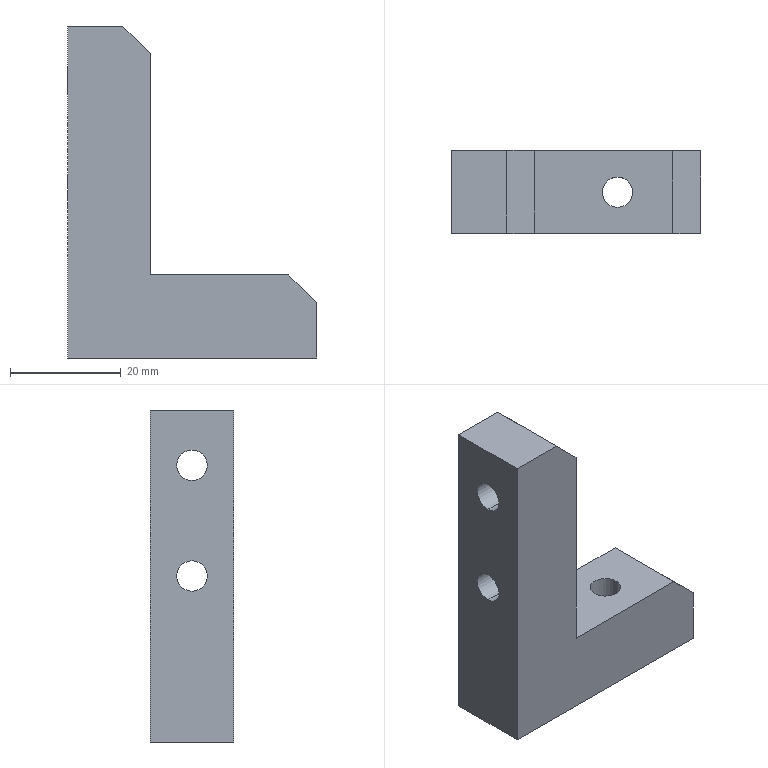Part | SolidWorks | features HoleWzd 2, Chamfer 1, Extrusion 1 | 1 solid | 16 faces | box 45 x 15 x 60 mm | volume 18806 mm3 | plane 10 | cylinder 6 | commonest cylinder face diameters 5.5 x6
STEP:
#1=CARTESIAN_POINT('',(12.25,0.,-15.));
#2=VERTEX_POINT('',#1);
#3=CARTESIAN_POINT('',(17.75,0.,-15.));
#4=VERTEX_POINT('',#3);
#5=CARTESIAN_POINT('',(15.,0.,-15.));
#6=DIRECTION('',(0.,0.,1.));
#7=DIRECTION('',(1.,0.,0.));
#8=AXIS2_PLACEMENT_3D('',#5,#6,#7);
#9=CIRCLE('',#8,2.75);
#10=EDGE_CURVE('',#2,#4,#9,.T.);
#11=ORIENTED_EDGE('',*,*,#10,.F.);
#12=CARTESIAN_POINT('',(12.25,0.,0.));
#13=VERTEX_POINT('',#12);
#14=CARTESIAN_POINT('',(12.25,0.,0.));
#15=DIRECTION('',(0.,0.,1.));
#16=VECTOR('',#15,1000.);
#17=LINE('',#14,#16);
#18=EDGE_CURVE('',#2,#13,#17,.T.);
#19=ORIENTED_EDGE('',*,*,#18,.T.);
#20=CARTESIAN_POINT('',(17.75,0.,0.));
#21=VERTEX_POINT('',#20);
#22=CARTESIAN_POINT('',(15.,0.,0.));
#23=DIRECTION('',(0.,0.,1.));
#24=DIRECTION('',(1.,0.,0.));
#25=AXIS2_PLACEMENT_3D('',#22,#23,#24);
#26=CIRCLE('',#25,2.75);
#27=EDGE_CURVE('',#13,#21,#26,.T.);
#28=ORIENTED_EDGE('',*,*,#27,.T.);
#29=CARTESIAN_POINT('',(17.75,0.,0.));
#30=DIRECTION('',(0.,0.,1.));
#31=VECTOR('',#30,1000.);
#32=LINE('',#29,#31);
#33=EDGE_CURVE('',#4,#21,#32,.T.);
#34=ORIENTED_EDGE('',*,*,#33,.F.);
#35=EDGE_LOOP('',(#11,#19,#28,#34));
#36=FACE_OUTER_BOUND('',#35,.T.);
#37=CARTESIAN_POINT('',(15.,0.,0.));
#38=DIRECTION('',(0.,0.,1.));
#39=DIRECTION('',(1.,0.,0.));
#40=AXIS2_PLACEMENT_3D('',#37,#38,#39);
#41=CYLINDRICAL_SURFACE('',#40,2.75);
#42=ADVANCED_FACE('',(#36),#41,.F.);
#43=CARTESIAN_POINT('',(-15.,0.,37.75));
#44=VERTEX_POINT('',#43);
#45=CARTESIAN_POINT('',(-15.,0.,32.25));
#46=VERTEX_POINT('',#45);
#47=CARTESIAN_POINT('',(-15.,0.,35.));
#48=DIRECTION('',(1.,0.,0.));
#49=DIRECTION('',(0.,0.,-1.));
#50=AXIS2_PLACEMENT_3D('',#47,#48,#49);
#51=CIRCLE('',#50,2.75);
#52=EDGE_CURVE('',#44,#46,#51,.T.);
#53=ORIENTED_EDGE('',*,*,#52,.F.);
#54=CARTESIAN_POINT('',(0.,0.,37.75));
#55=VERTEX_POINT('',#54);
#56=CARTESIAN_POINT('',(0.,0.,37.75));
#57=DIRECTION('',(1.,0.,0.));
#58=VECTOR('',#57,1000.);
#59=LINE('',#56,#58);
#60=EDGE_CURVE('',#44,#55,#59,.T.);
#61=ORIENTED_EDGE('',*,*,#60,.T.);
#62=CARTESIAN_POINT('',(0.,0.,32.25));
#63=VERTEX_POINT('',#62);
#64=CARTESIAN_POINT('',(0.,0.,35.));
#65=DIRECTION('',(1.,0.,0.));
#66=DIRECTION('',(0.,0.,-1.));
#67=AXIS2_PLACEMENT_3D('',#64,#65,#66);
#68=CIRCLE('',#67,2.75);
#69=EDGE_CURVE('',#55,#63,#68,.T.);
#70=ORIENTED_EDGE('',*,*,#69,.T.);
#71=CARTESIAN_POINT('',(0.,0.,32.25));
#72=DIRECTION('',(1.,0.,0.));
#73=VECTOR('',#72,1000.);
#74=LINE('',#71,#73);
#75=EDGE_CURVE('',#46,#63,#74,.T.);
#76=ORIENTED_EDGE('',*,*,#75,.F.);
#77=EDGE_LOOP('',(#53,#61,#70,#76));
#78=FACE_OUTER_BOUND('',#77,.T.);
#79=CARTESIAN_POINT('',(0.,0.,35.));
#80=DIRECTION('',(1.,0.,0.));
#81=DIRECTION('',(0.,0.,-1.));
#82=AXIS2_PLACEMENT_3D('',#79,#80,#81);
#83=CYLINDRICAL_SURFACE('',#82,2.75);
#84=ADVANCED_FACE('',(#78),#83,.F.);
#85=CARTESIAN_POINT('',(-15.,0.,17.75));
#86=VERTEX_POINT('',#85);
#87=CARTESIAN_POINT('',(-15.,0.,12.25));
#88=VERTEX_POINT('',#87);
#89=CARTESIAN_POINT('',(-15.,0.,15.));
#90=DIRECTION('',(1.,0.,0.));
#91=DIRECTION('',(0.,0.,-1.));
#92=AXIS2_PLACEMENT_3D('',#89,#90,#91);
#93=CIRCLE('',#92,2.75);
#94=EDGE_CURVE('',#86,#88,#93,.T.);
#95=ORIENTED_EDGE('',*,*,#94,.F.);
#96=CARTESIAN_POINT('',(0.,0.,17.75));
#97=VERTEX_POINT('',#96);
#98=CARTESIAN_POINT('',(0.,0.,17.75));
#99=DIRECTION('',(1.,0.,0.));
#100=VECTOR('',#99,1000.);
#101=LINE('',#98,#100);
#102=EDGE_CURVE('',#86,#97,#101,.T.);
#103=ORIENTED_EDGE('',*,*,#102,.T.);
#104=CARTESIAN_POINT('',(0.,0.,12.25));
#105=VERTEX_POINT('',#104);
#106=CARTESIAN_POINT('',(0.,0.,15.));
#107=DIRECTION('',(1.,0.,0.));
#108=DIRECTION('',(0.,0.,-1.));
#109=AXIS2_PLACEMENT_3D('',#106,#107,#108);
#110=CIRCLE('',#109,2.75);
#111=EDGE_CURVE('',#97,#105,#110,.T.);
#112=ORIENTED_EDGE('',*,*,#111,.T.);
#113=CARTESIAN_POINT('',(0.,0.,12.25));
#114=DIRECTION('',(1.,0.,0.));
#115=VECTOR('',#114,1000.);
#116=LINE('',#113,#115);
#117=EDGE_CURVE('',#88,#105,#116,.T.);
#118=ORIENTED_EDGE('',*,*,#117,.F.);
#119=EDGE_LOOP('',(#95,#103,#112,#118));
#120=FACE_OUTER_BOUND('',#119,.T.);
#121=CARTESIAN_POINT('',(0.,0.,15.));
#122=DIRECTION('',(1.,0.,0.));
#123=DIRECTION('',(0.,0.,-1.));
#124=AXIS2_PLACEMENT_3D('',#121,#122,#123);
#125=CYLINDRICAL_SURFACE('',#124,2.75);
#126=ADVANCED_FACE('',(#120),#125,.F.);
#127=CARTESIAN_POINT('',(-15.,0.,35.));
#128=DIRECTION('',(1.,0.,0.));
#129=DIRECTION('',(0.,0.,-1.));
#130=AXIS2_PLACEMENT_3D('',#127,#128,#129);
#131=CIRCLE('',#130,2.75);
#132=EDGE_CURVE('',#46,#44,#131,.T.);
#133=ORIENTED_EDGE('',*,*,#132,.T.);
#134=ORIENTED_EDGE('',*,*,#52,.T.);
#135=EDGE_LOOP('',(#133,#134));
#136=FACE_BOUND('',#135,.T.);
#137=CARTESIAN_POINT('',(-15.,0.,15.));
#138=DIRECTION('',(1.,0.,0.));
#139=DIRECTION('',(0.,0.,-1.));
#140=AXIS2_PLACEMENT_3D('',#137,#138,#139);
#141=CIRCLE('',#140,2.75);
#142=EDGE_CURVE('',#88,#86,#141,.T.);
#143=ORIENTED_EDGE('',*,*,#142,.T.);
#144=ORIENTED_EDGE('',*,*,#94,.T.);
#145=EDGE_LOOP('',(#143,#144));
#146=FACE_BOUND('',#145,.T.);
#147=CARTESIAN_POINT('',(-15.,-7.5,-15.));
#148=VERTEX_POINT('',#147);
#149=CARTESIAN_POINT('',(-15.,-7.5,45.));
#150=VERTEX_POINT('',#149);
#151=CARTESIAN_POINT('',(-15.,-7.5,-15.));
#152=DIRECTION('',(0.,0.,1.));
#153=VECTOR('',#152,1000.);
#154=LINE('',#151,#153);
#155=EDGE_CURVE('',#148,#150,#154,.T.);
#156=ORIENTED_EDGE('',*,*,#155,.T.);
#157=CARTESIAN_POINT('',(-15.,7.5,45.));
#158=VERTEX_POINT('',#157);
#159=CARTESIAN_POINT('',(-15.,7.5,45.));
#160=DIRECTION('',(0.,-1.,0.));
#161=VECTOR('',#160,1000.);
#162=LINE('',#159,#161);
#163=EDGE_CURVE('',#158,#150,#162,.T.);
#164=ORIENTED_EDGE('',*,*,#163,.F.);
#165=CARTESIAN_POINT('',(-15.,7.5,-15.));
#166=VERTEX_POINT('',#165);
#167=CARTESIAN_POINT('',(-15.,7.5,-15.));
#168=DIRECTION('',(0.,0.,1.));
#169=VECTOR('',#168,1000.);
#170=LINE('',#167,#169);
#171=EDGE_CURVE('',#166,#158,#170,.T.);
#172=ORIENTED_EDGE('',*,*,#171,.F.);
#173=CARTESIAN_POINT('',(-15.,7.5,-15.));
#174=DIRECTION('',(0.,-1.,0.));
#175=VECTOR('',#174,1000.);
#176=LINE('',#173,#175);
#177=EDGE_CURVE('',#166,#148,#176,.T.);
#178=ORIENTED_EDGE('',*,*,#177,.T.);
#179=EDGE_LOOP('',(#156,#164,#172,#178));
#180=FACE_OUTER_BOUND('',#179,.T.);
#181=CARTESIAN_POINT('',(-15.,7.5,-15.));
#182=DIRECTION('',(1.,0.,0.));
#183=DIRECTION('',(0.,0.,-1.));
#184=AXIS2_PLACEMENT_3D('',#181,#182,#183);
#185=PLANE('',#184);
#186=ADVANCED_FACE('',(#136,#146,#180),#185,.F.);
#187=CARTESIAN_POINT('',(-5.,-7.5,45.));
#188=VERTEX_POINT('',#187);
#189=CARTESIAN_POINT('',(0.,-7.5,45.));
#190=DIRECTION('',(1.,0.,0.));
#191=VECTOR('',#190,1000.);
#192=LINE('',#189,#191);
#193=EDGE_CURVE('',#150,#188,#192,.T.);
#194=ORIENTED_EDGE('',*,*,#193,.T.);
#195=CARTESIAN_POINT('',(-5.,7.5,45.));
#196=VERTEX_POINT('',#195);
#197=CARTESIAN_POINT('',(-5.,7.5,45.));
#198=DIRECTION('',(0.,1.,0.));
#199=VECTOR('',#198,1000.);
#200=LINE('',#197,#199);
#201=EDGE_CURVE('',#188,#196,#200,.T.);
#202=ORIENTED_EDGE('',*,*,#201,.T.);
#203=CARTESIAN_POINT('',(0.,7.5,45.));
#204=DIRECTION('',(1.,0.,0.));
#205=VECTOR('',#204,1000.);
#206=LINE('',#203,#205);
#207=EDGE_CURVE('',#158,#196,#206,.T.);
#208=ORIENTED_EDGE('',*,*,#207,.F.);
#209=ORIENTED_EDGE('',*,*,#163,.T.);
#210=EDGE_LOOP('',(#194,#202,#208,#209));
#211=FACE_OUTER_BOUND('',#210,.T.);
#212=CARTESIAN_POINT('',(0.,7.5,45.));
#213=DIRECTION('',(0.,0.,-1.));
#214=DIRECTION('',(-1.,0.,0.));
#215=AXIS2_PLACEMENT_3D('',#212,#213,#214);
#216=PLANE('',#215);
#217=ADVANCED_FACE('',(#211),#216,.F.);
#218=CARTESIAN_POINT('',(0.,0.,35.));
#219=DIRECTION('',(1.,0.,0.));
#220=DIRECTION('',(0.,0.,-1.));
#221=AXIS2_PLACEMENT_3D('',#218,#219,#220);
#222=CIRCLE('',#221,2.75);
#223=EDGE_CURVE('',#63,#55,#222,.T.);
#224=ORIENTED_EDGE('',*,*,#223,.F.);
#225=ORIENTED_EDGE('',*,*,#69,.F.);
#226=EDGE_LOOP('',(#224,#225));
#227=FACE_BOUND('',#226,.T.);
#228=CARTESIAN_POINT('',(0.,0.,15.));
#229=DIRECTION('',(1.,0.,0.));
#230=DIRECTION('',(0.,0.,-1.));
#231=AXIS2_PLACEMENT_3D('',#228,#229,#230);
#232=CIRCLE('',#231,2.75);
#233=EDGE_CURVE('',#105,#97,#232,.T.);
#234=ORIENTED_EDGE('',*,*,#233,.F.);
#235=ORIENTED_EDGE('',*,*,#111,.F.);
#236=EDGE_LOOP('',(#234,#235));
#237=FACE_BOUND('',#236,.T.);
#238=CARTESIAN_POINT('',(0.,7.5,40.));
#239=VERTEX_POINT('',#238);
#240=CARTESIAN_POINT('',(0.,7.5,0.));
#241=VERTEX_POINT('',#240);
#242=CARTESIAN_POINT('',(0.,7.5,0.));
#243=DIRECTION('',(0.,0.,-1.));
#244=VECTOR('',#243,1000.);
#245=LINE('',#242,#244);
#246=EDGE_CURVE('',#239,#241,#245,.T.);
#247=ORIENTED_EDGE('',*,*,#246,.F.);
#248=CARTESIAN_POINT('',(0.,-7.5,40.));
#249=VERTEX_POINT('',#248);
#250=CARTESIAN_POINT('',(0.,7.5,40.));
#251=DIRECTION('',(0.,-1.,0.));
#252=VECTOR('',#251,1000.);
#253=LINE('',#250,#252);
#254=EDGE_CURVE('',#239,#249,#253,.T.);
#255=ORIENTED_EDGE('',*,*,#254,.T.);
#256=CARTESIAN_POINT('',(0.,-7.5,0.));
#257=VERTEX_POINT('',#256);
#258=CARTESIAN_POINT('',(0.,-7.5,0.));
#259=DIRECTION('',(0.,0.,-1.));
#260=VECTOR('',#259,1000.);
#261=LINE('',#258,#260);
#262=EDGE_CURVE('',#249,#257,#261,.T.);
#263=ORIENTED_EDGE('',*,*,#262,.T.);
#264=CARTESIAN_POINT('',(0.,7.5,0.));
#265=DIRECTION('',(0.,-1.,0.));
#266=VECTOR('',#265,1000.);
#267=LINE('',#264,#266);
#268=EDGE_CURVE('',#241,#257,#267,.T.);
#269=ORIENTED_EDGE('',*,*,#268,.F.);
#270=EDGE_LOOP('',(#247,#255,#263,#269));
#271=FACE_OUTER_BOUND('',#270,.T.);
#272=CARTESIAN_POINT('',(0.,7.5,0.));
#273=DIRECTION('',(-1.,0.,0.));
#274=DIRECTION('',(0.,0.,1.));
#275=AXIS2_PLACEMENT_3D('',#272,#273,#274);
#276=PLANE('',#275);
#277=ADVANCED_FACE('',(#227,#237,#271),#276,.F.);
#278=CARTESIAN_POINT('',(15.,0.,0.));
#279=DIRECTION('',(0.,0.,1.));
#280=DIRECTION('',(1.,0.,0.));
#281=AXIS2_PLACEMENT_3D('',#278,#279,#280);
#282=CIRCLE('',#281,2.75);
#283=EDGE_CURVE('',#21,#13,#282,.T.);
#284=ORIENTED_EDGE('',*,*,#283,.F.);
#285=ORIENTED_EDGE('',*,*,#27,.F.);
#286=EDGE_LOOP('',(#284,#285));
#287=FACE_BOUND('',#286,.T.);
#288=CARTESIAN_POINT('',(25.,-7.5,0.));
#289=VERTEX_POINT('',#288);
#290=CARTESIAN_POINT('',(30.,-7.5,0.));
#291=DIRECTION('',(1.,0.,0.));
#292=VECTOR('',#291,1000.);
#293=LINE('',#290,#292);
#294=EDGE_CURVE('',#257,#289,#293,.T.);
#295=ORIENTED_EDGE('',*,*,#294,.T.);
#296=CARTESIAN_POINT('',(25.,7.5,0.));
#297=VERTEX_POINT('',#296);
#298=CARTESIAN_POINT('',(25.,7.5,0.));
#299=DIRECTION('',(0.,1.,0.));
#300=VECTOR('',#299,1000.);
#301=LINE('',#298,#300);
#302=EDGE_CURVE('',#289,#297,#301,.T.);
#303=ORIENTED_EDGE('',*,*,#302,.T.);
#304=CARTESIAN_POINT('',(30.,7.5,0.));
#305=DIRECTION('',(1.,0.,0.));
#306=VECTOR('',#305,1000.);
#307=LINE('',#304,#306);
#308=EDGE_CURVE('',#241,#297,#307,.T.);
#309=ORIENTED_EDGE('',*,*,#308,.F.);
#310=ORIENTED_EDGE('',*,*,#268,.T.);
#311=EDGE_LOOP('',(#295,#303,#309,#310));
#312=FACE_OUTER_BOUND('',#311,.T.);
#313=CARTESIAN_POINT('',(30.,7.5,0.));
#314=DIRECTION('',(0.,0.,-1.));
#315=DIRECTION('',(-1.,0.,0.));
#316=AXIS2_PLACEMENT_3D('',#313,#314,#315);
#317=PLANE('',#316);
#318=ADVANCED_FACE('',(#287,#312),#317,.F.);
#319=CARTESIAN_POINT('',(30.,7.5,-5.));
#320=VERTEX_POINT('',#319);
#321=CARTESIAN_POINT('',(30.,7.5,-15.));
#322=VERTEX_POINT('',#321);
#323=CARTESIAN_POINT('',(30.,7.5,-15.));
#324=DIRECTION('',(0.,0.,-1.));
#325=VECTOR('',#324,1000.);
#326=LINE('',#323,#325);
#327=EDGE_CURVE('',#320,#322,#326,.T.);
#328=ORIENTED_EDGE('',*,*,#327,.F.);
#329=CARTESIAN_POINT('',(30.,-7.5,-5.));
#330=VERTEX_POINT('',#329);
#331=CARTESIAN_POINT('',(30.,7.5,-5.));
#332=DIRECTION('',(0.,-1.,0.));
#333=VECTOR('',#332,1000.);
#334=LINE('',#331,#333);
#335=EDGE_CURVE('',#320,#330,#334,.T.);
#336=ORIENTED_EDGE('',*,*,#335,.T.);
#337=CARTESIAN_POINT('',(30.,-7.5,-15.));
#338=VERTEX_POINT('',#337);
#339=CARTESIAN_POINT('',(30.,-7.5,-15.));
#340=DIRECTION('',(0.,0.,-1.));
#341=VECTOR('',#340,1000.);
#342=LINE('',#339,#341);
#343=EDGE_CURVE('',#330,#338,#342,.T.);
#344=ORIENTED_EDGE('',*,*,#343,.T.);
#345=CARTESIAN_POINT('',(30.,7.5,-15.));
#346=DIRECTION('',(0.,-1.,0.));
#347=VECTOR('',#346,1000.);
#348=LINE('',#345,#347);
#349=EDGE_CURVE('',#322,#338,#348,.T.);
#350=ORIENTED_EDGE('',*,*,#349,.F.);
#351=EDGE_LOOP('',(#328,#336,#344,#350));
#352=FACE_OUTER_BOUND('',#351,.T.);
#353=CARTESIAN_POINT('',(30.,7.5,-15.));
#354=DIRECTION('',(-1.,0.,0.));
#355=DIRECTION('',(0.,0.,1.));
#356=AXIS2_PLACEMENT_3D('',#353,#354,#355);
#357=PLANE('',#356);
#358=ADVANCED_FACE('',(#352),#357,.F.);
#359=CARTESIAN_POINT('',(15.,0.,-15.));
#360=DIRECTION('',(0.,0.,1.));
#361=DIRECTION('',(1.,0.,0.));
#362=AXIS2_PLACEMENT_3D('',#359,#360,#361);
#363=CIRCLE('',#362,2.75);
#364=EDGE_CURVE('',#4,#2,#363,.T.);
#365=ORIENTED_EDGE('',*,*,#364,.T.);
#366=ORIENTED_EDGE('',*,*,#10,.T.);
#367=EDGE_LOOP('',(#365,#366));
#368=FACE_BOUND('',#367,.T.);
#369=CARTESIAN_POINT('',(30.,-7.5,-15.));
#370=DIRECTION('',(-1.,0.,0.));
#371=VECTOR('',#370,1000.);
#372=LINE('',#369,#371);
#373=EDGE_CURVE('',#338,#148,#372,.T.);
#374=ORIENTED_EDGE('',*,*,#373,.T.);
#375=ORIENTED_EDGE('',*,*,#177,.F.);
#376=CARTESIAN_POINT('',(30.,7.5,-15.));
#377=DIRECTION('',(-1.,0.,0.));
#378=VECTOR('',#377,1000.);
#379=LINE('',#376,#378);
#380=EDGE_CURVE('',#322,#166,#379,.T.);
#381=ORIENTED_EDGE('',*,*,#380,.F.);
#382=ORIENTED_EDGE('',*,*,#349,.T.);
#383=EDGE_LOOP('',(#374,#375,#381,#382));
#384=FACE_OUTER_BOUND('',#383,.T.);
#385=CARTESIAN_POINT('',(30.,7.5,-15.));
#386=DIRECTION('',(0.,0.,1.));
#387=DIRECTION('',(1.,0.,0.));
#388=AXIS2_PLACEMENT_3D('',#385,#386,#387);
#389=PLANE('',#388);
#390=ADVANCED_FACE('',(#368,#384),#389,.F.);
#391=ORIENTED_EDGE('',*,*,#207,.T.);
#392=CARTESIAN_POINT('',(0.,7.5,40.));
#393=DIRECTION('',(0.7071,0.,-0.7071));
#394=VECTOR('',#393,1000.);
#395=LINE('',#392,#394);
#396=EDGE_CURVE('',#196,#239,#395,.T.);
#397=ORIENTED_EDGE('',*,*,#396,.T.);
#398=ORIENTED_EDGE('',*,*,#246,.T.);
#399=ORIENTED_EDGE('',*,*,#308,.T.);
#400=CARTESIAN_POINT('',(30.,7.5,-5.));
#401=DIRECTION('',(0.7071,0.,-0.7071));
#402=VECTOR('',#401,1000.);
#403=LINE('',#400,#402);
#404=EDGE_CURVE('',#297,#320,#403,.T.);
#405=ORIENTED_EDGE('',*,*,#404,.T.);
#406=ORIENTED_EDGE('',*,*,#327,.T.);
#407=ORIENTED_EDGE('',*,*,#380,.T.);
#408=ORIENTED_EDGE('',*,*,#171,.T.);
#409=EDGE_LOOP('',(#391,#397,#398,#399,#405,#406,#407,#408));
#410=FACE_OUTER_BOUND('',#409,.T.);
#411=CARTESIAN_POINT('',(0.,7.5,0.));
#412=DIRECTION('',(0.,-1.,0.));
#413=DIRECTION('',(0.,0.,-1.));
#414=AXIS2_PLACEMENT_3D('',#411,#412,#413);
#415=PLANE('',#414);
#416=ADVANCED_FACE('',(#410),#415,.F.);
#417=ORIENTED_EDGE('',*,*,#262,.F.);
#418=CARTESIAN_POINT('',(20.,-7.5,20.));
#419=DIRECTION('',(-0.7071,0.,0.7071));
#420=VECTOR('',#419,1000.);
#421=LINE('',#418,#420);
#422=EDGE_CURVE('',#249,#188,#421,.T.);
#423=ORIENTED_EDGE('',*,*,#422,.T.);
#424=ORIENTED_EDGE('',*,*,#193,.F.);
#425=ORIENTED_EDGE('',*,*,#155,.F.);
#426=ORIENTED_EDGE('',*,*,#373,.F.);
#427=ORIENTED_EDGE('',*,*,#343,.F.);
#428=CARTESIAN_POINT('',(12.5,-7.5,12.5));
#429=DIRECTION('',(-0.7071,0.,0.7071));
#430=VECTOR('',#429,1000.);
#431=LINE('',#428,#430);
#432=EDGE_CURVE('',#330,#289,#431,.T.);
#433=ORIENTED_EDGE('',*,*,#432,.T.);
#434=ORIENTED_EDGE('',*,*,#294,.F.);
#435=EDGE_LOOP('',(#417,#423,#424,#425,#426,#427,#433,#434));
#436=FACE_OUTER_BOUND('',#435,.T.);
#437=CARTESIAN_POINT('',(0.,-7.5,0.));
#438=DIRECTION('',(0.,-1.,0.));
#439=DIRECTION('',(0.,0.,-1.));
#440=AXIS2_PLACEMENT_3D('',#437,#438,#439);
#441=PLANE('',#440);
#442=ADVANCED_FACE('',(#436),#441,.T.);
#443=ORIENTED_EDGE('',*,*,#396,.F.);
#444=ORIENTED_EDGE('',*,*,#201,.F.);
#445=ORIENTED_EDGE('',*,*,#422,.F.);
#446=ORIENTED_EDGE('',*,*,#254,.F.);
#447=EDGE_LOOP('',(#443,#444,#445,#446));
#448=FACE_OUTER_BOUND('',#447,.T.);
#449=CARTESIAN_POINT('',(0.,7.5,40.));
#450=DIRECTION('',(-0.7071,0.,-0.7071));
#451=DIRECTION('',(0.,-1.,0.));
#452=AXIS2_PLACEMENT_3D('',#449,#450,#451);
#453=PLANE('',#452);
#454=ADVANCED_FACE('',(#448),#453,.F.);
#455=ORIENTED_EDGE('',*,*,#404,.F.);
#456=ORIENTED_EDGE('',*,*,#302,.F.);
#457=ORIENTED_EDGE('',*,*,#432,.F.);
#458=ORIENTED_EDGE('',*,*,#335,.F.);
#459=EDGE_LOOP('',(#455,#456,#457,#458));
#460=FACE_OUTER_BOUND('',#459,.T.);
#461=CARTESIAN_POINT('',(30.,7.5,-5.));
#462=DIRECTION('',(-0.7071,0.,-0.7071));
#463=DIRECTION('',(0.,-1.,0.));
#464=AXIS2_PLACEMENT_3D('',#461,#462,#463);
#465=PLANE('',#464);
#466=ADVANCED_FACE('',(#460),#465,.F.);
#467=ORIENTED_EDGE('',*,*,#102,.F.);
#468=ORIENTED_EDGE('',*,*,#142,.F.);
#469=ORIENTED_EDGE('',*,*,#117,.T.);
#470=ORIENTED_EDGE('',*,*,#233,.T.);
#471=EDGE_LOOP('',(#467,#468,#469,#470));
#472=FACE_OUTER_BOUND('',#471,.T.);
#473=CARTESIAN_POINT('',(0.,0.,15.));
#474=DIRECTION('',(1.,0.,0.));
#475=DIRECTION('',(0.,0.,-1.));
#476=AXIS2_PLACEMENT_3D('',#473,#474,#475);
#477=CYLINDRICAL_SURFACE('',#476,2.75);
#478=ADVANCED_FACE('',(#472),#477,.F.);
#479=ORIENTED_EDGE('',*,*,#60,.F.);
#480=ORIENTED_EDGE('',*,*,#132,.F.);
#481=ORIENTED_EDGE('',*,*,#75,.T.);
#482=ORIENTED_EDGE('',*,*,#223,.T.);
#483=EDGE_LOOP('',(#479,#480,#481,#482));
#484=FACE_OUTER_BOUND('',#483,.T.);
#485=CARTESIAN_POINT('',(0.,0.,35.));
#486=DIRECTION('',(1.,0.,0.));
#487=DIRECTION('',(0.,0.,-1.));
#488=AXIS2_PLACEMENT_3D('',#485,#486,#487);
#489=CYLINDRICAL_SURFACE('',#488,2.75);
#490=ADVANCED_FACE('',(#484),#489,.F.);
#491=ORIENTED_EDGE('',*,*,#18,.F.);
#492=ORIENTED_EDGE('',*,*,#364,.F.);
#493=ORIENTED_EDGE('',*,*,#33,.T.);
#494=ORIENTED_EDGE('',*,*,#283,.T.);
#495=EDGE_LOOP('',(#491,#492,#493,#494));
#496=FACE_OUTER_BOUND('',#495,.T.);
#497=CARTESIAN_POINT('',(15.,0.,0.));
#498=DIRECTION('',(0.,0.,1.));
#499=DIRECTION('',(1.,0.,0.));
#500=AXIS2_PLACEMENT_3D('',#497,#498,#499);
#501=CYLINDRICAL_SURFACE('',#500,2.75);
#502=ADVANCED_FACE('',(#496),#501,.F.);
#503=CLOSED_SHELL('',(#42,#84,#126,#186,#217,#277,#318,#358,#390,#416,#442,#454,#466,#478,#490,#502));
#504=MANIFOLD_SOLID_BREP('',#503);
#505=CARTESIAN_POINT('',(0.,0.,0.));
#506=DIRECTION('',(0.,0.,1.));
#507=DIRECTION('',(1.,0.,0.));
#508=AXIS2_PLACEMENT_3D('',#505,#506,#507);
#509=(LENGTH_UNIT()NAMED_UNIT(*)SI_UNIT(.MILLI.,.METRE.));
#510=UNCERTAINTY_MEASURE_WITH_UNIT(LENGTH_MEASURE(0.00001),#509,'','');
#511=(NAMED_UNIT(*)PLANE_ANGLE_UNIT()SI_UNIT($,.RADIAN.));
#512=(NAMED_UNIT(*)SI_UNIT($,.STERADIAN.)SOLID_ANGLE_UNIT());
#513=(GEOMETRIC_REPRESENTATION_CONTEXT(3)GLOBAL_UNCERTAINTY_ASSIGNED_CONTEXT((#510))GLOBAL_UNIT_ASSIGNED_CONTEXT((#509,#511,#512))REPRESENTATION_CONTEXT('',''));
#514=ADVANCED_BREP_SHAPE_REPRESENTATION('',(#504,#508),#513);